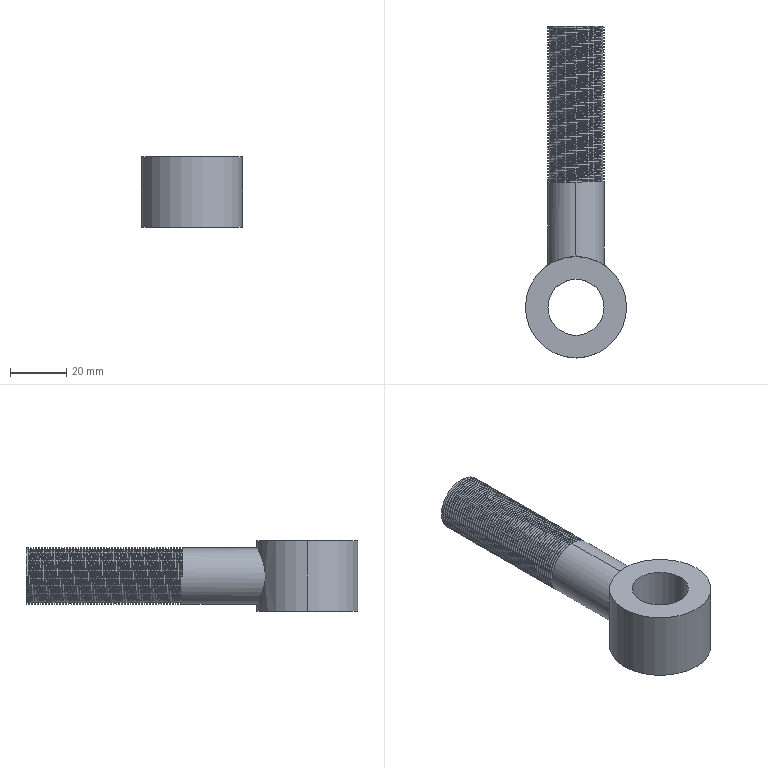Part | SolidWorks | features Extrusion 1, Revolution 1, SweepThread 1 | 1 solid | 124 faces | box 36 x 118 x 25 mm | volume 42808 mm3 | cylinder 116 | plane 5 | spline 3 | commonest cylinder face diameters 20 x114 36 x2